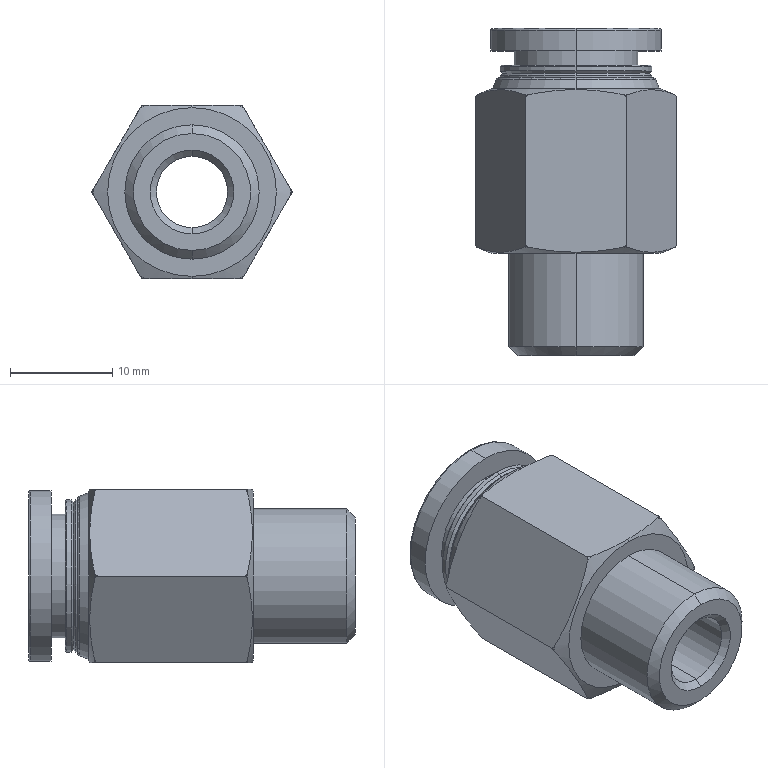Part | STEP file | BPC1002 | 1 solid | 62 faces | box 19.63 x 32 x 17 mm | volume 3663 mm3 | torus 18 | cone 16 | cylinder 14 | plane 14 | commonest cylinder face diameters 14.9 x4 7 x2 12 x2 12.1 x2 13.157 x2 16.7 x2